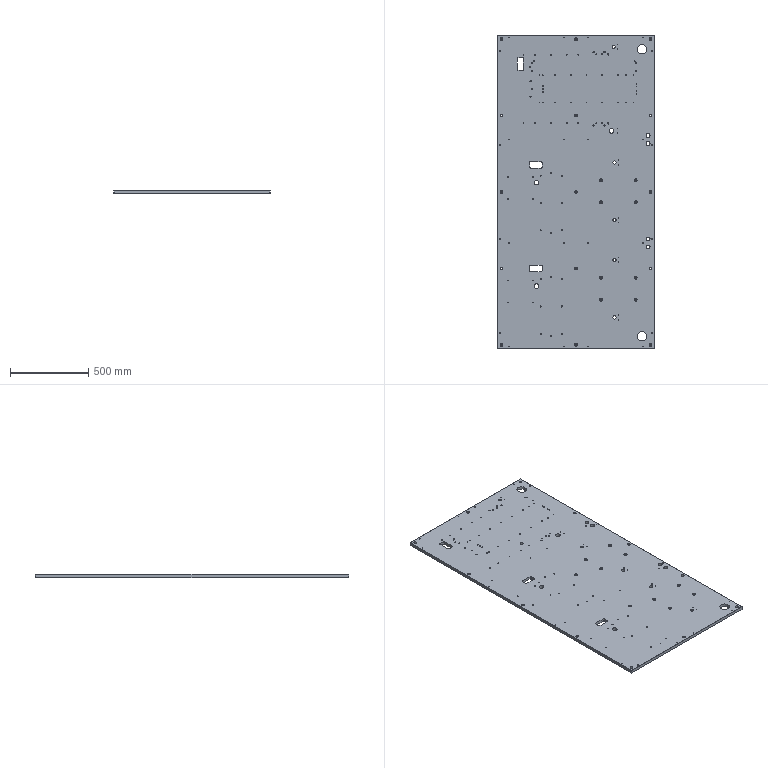Part | SolidWorks | features HoleWzd 18, Cut 5, Chamfer 2, Extrusion 1, Fillet 1, ICE 1, MirrorPattern 1 | 1 solid | 605 faces | box 1000 x 2000 x 20 mm | volume 39453468 mm3 | cylinder 362 | cone 190 | plane 53 | commonest cylinder face diameters 5 x120 6.8 x40 6 x34 11 x30 18 x30 20 x26